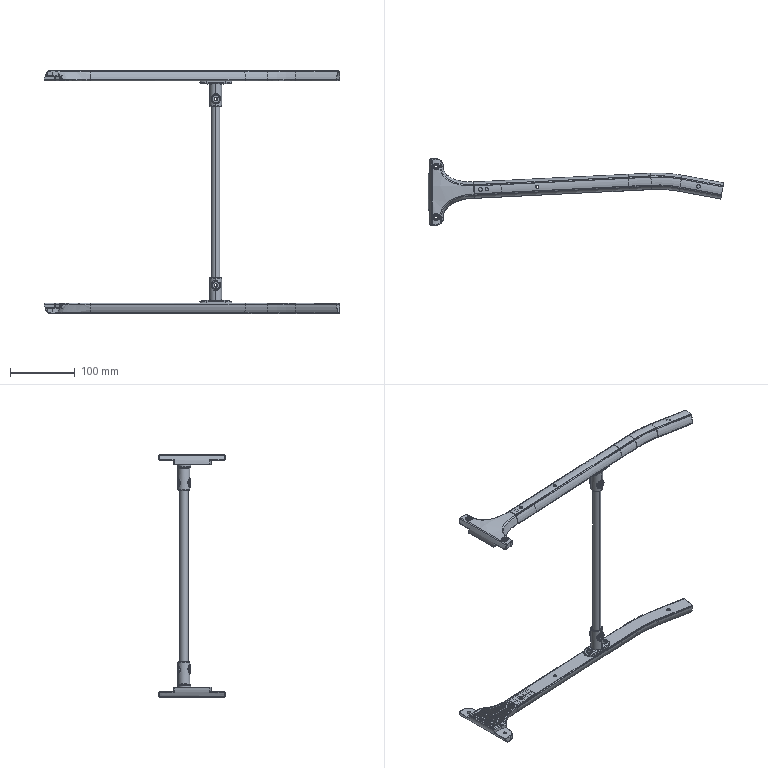Part | SolidWorks | 7 solids | 1434 faces | box 457.689 x 102.814 x 377.765 mm | volume 176220 mm3 | plane 582 | cylinder 437 | spline 403 | torus 6 | cone 6 | commonest cylinder face diameters 5.2 x48 2.745 x33 0.98 x22 5.882 x20 41.765 x20 0.6 x16